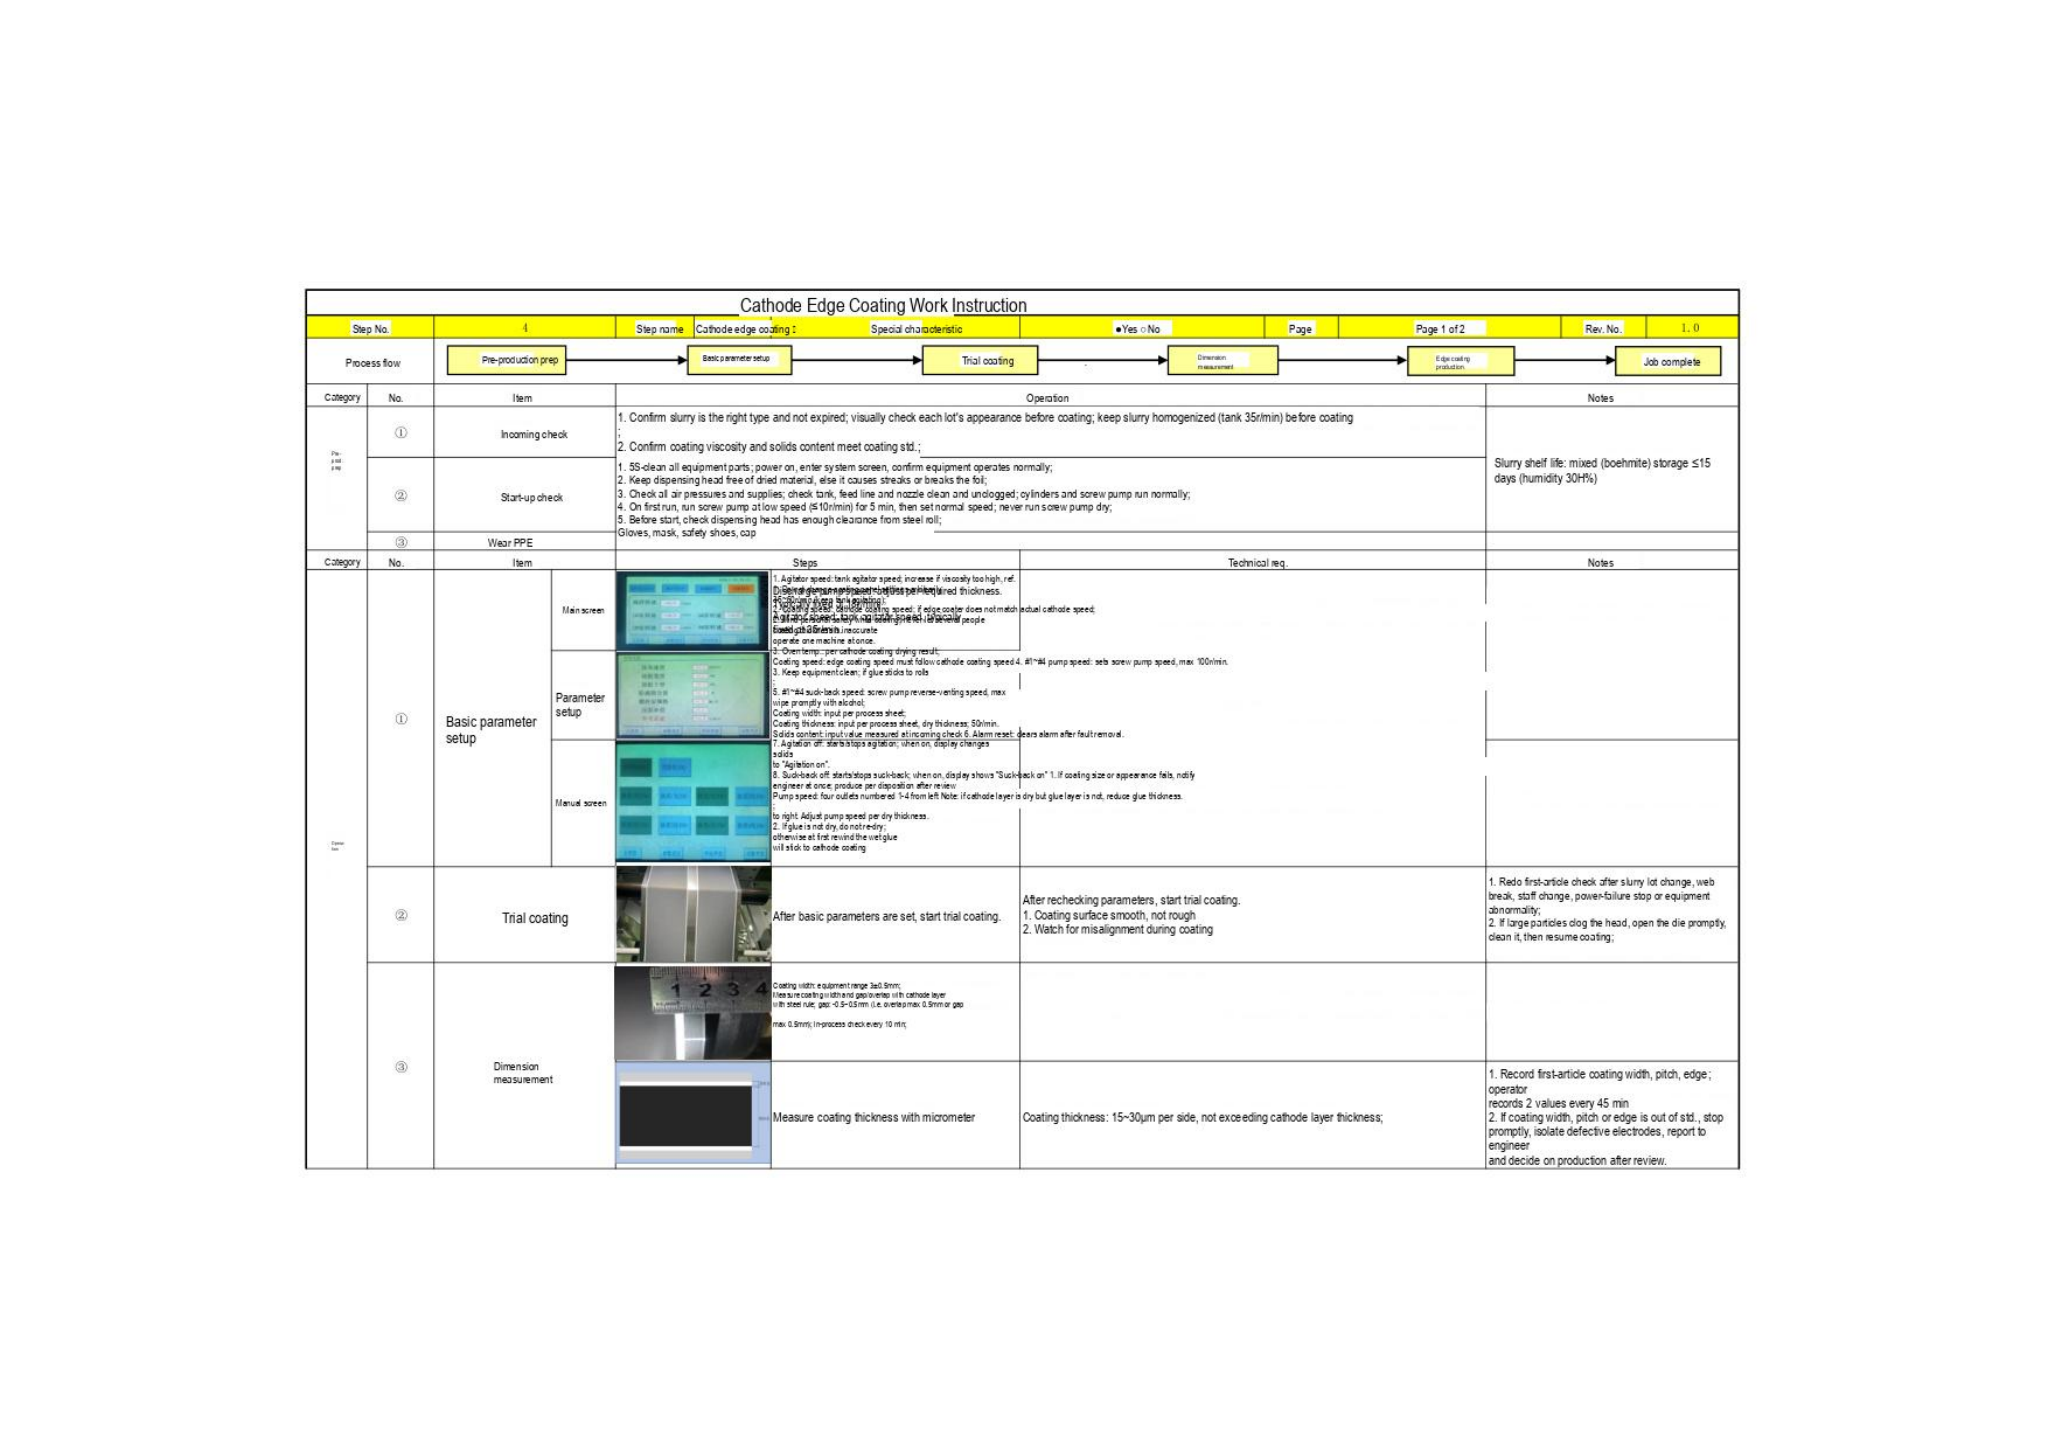# Cathode Edge Coating Work Instruction

| Step No. | 4 | Step name | Cathode edge coating | Special characteristic | ●Yes ○No | Page | Page 1 of 2 | Rev. No. | 1.0 |
|---|---|---|---|---|---|---|---|---|---|

Process flow: Pre-production prep → Basic parameter setup → Trial coating → Dimension measurement → Edge coating production → Job complete

| Category | No. | Item | Operation | Notes |
|---|---|---|---|---|
| Pre-prod prep | ① | Incoming check | 1. Confirm slurry is the right type and not expired; visually check each lot's appearance before coating; keep slurry homogenized (tank 35r/min) before coating<br>;<br>2. Confirm coating viscosity and solids content meet coating std.; | Slurry shelf life: mixed (boehmite) storage ≤15 days (humidity 30H%) |
| | ② | Start-up check | 1. 5S-clean all equipment parts; power on, enter system screen, confirm equipment operates normally;<br>2. Keep dispensing head free of dried material, else it causes streaks or breaks the foil;<br>3. Check all air pressures and supplies; check tank, feed line and nozzle clean and unclogged; cylinders and screw pump run normally;<br>4. On first run, run screw pump at low speed (≤10r/min) for 5 min, then set normal speed; never run screw pump dry;<br>5. Before start, check dispensing head has enough clearance from steel roll; | |
| | ③ | Wear PPE | Gloves, mask, safety shoes, cap | |

| Category | No. | Item | | Steps | Technical req. | Notes |
|---|---|---|---|---|---|---|
| Operation | ① | Basic parameter setup | Main screen<br>Parameter setup<br>Manual screen | 1. Agitator speed: tank agitator speed; increase if viscosity too high, ref.<br>Dispense pump speed: adjust per required thickness.<br>2. Coating speed: cathode coating speed; if edge coater does not match actual cathode speed;<br>inaccurate<br>operate one machine at once.<br>3. Oven temp.: per cathode coating drying result;<br>Coating speed: edge coating speed must follow cathode coating speed 4. #1~#4 pump speed: sets screw pump speed, max 100r/min.<br>3. Keep equipment clean; if glue sticks to rolls<br>5. #1~#4 suck-back speed: screw pump reverse-venting speed, max<br>wipe promptly with alcohol;<br>Coating width: input per process sheet;<br>Coating thickness: input per process sheet, dry thickness; 50r/min.<br>Solids content: input value measured at incoming check 6. Alarm reset: clears alarm after fault removal.<br>7. Agitation off: starts/stops agitation; when on, display changes<br>solids<br>to "Agitation on".<br>8. Suck-back off: starts/stops suck-back; when on, display shows "Suck-back on" 1. If coating size or appearance fails, notify<br>engineer at once; produce per disposition after review<br>Pump speed: four outlets numbered 1-4 from left Note: if cathode layer is dry but glue layer is not, reduce glue thickness.<br>to right. Adjust pump speed per dry thickness.<br>2. If glue is not dry, do not re-dry;<br>otherwise at first rewind the wet glue<br>will stick to cathode coating | | |
| | ② | Trial coating | | After basic parameters are set, start trial coating. | After rechecking parameters, start trial coating.<br>1. Coating surface smooth, not rough<br>2. Watch for misalignment during coating | 1. Redo first-article check after slurry lot change, web break, staff change, power-failure stop or equipment abnormality;<br>2. If large particles clog the head, open the die promptly, clean it, then resume coating; |
| | ③ | Dimension measurement | | 1 2 3 4<br>Coating width: equipment range 3±0.5mm;<br>Measure coating width and gap/overlap with cathode layer with steel rule; gap: -0.5~0.5mm (i.e. overlap max 0.5mm or gap max 0.5mm); in-process check every 10 min; | | |
| | | | | Measure coating thickness with micrometer | Coating thickness: 15~30μm per side, not exceeding cathode layer thickness; | 1. Record first-article coating width, pitch, edge; operator records 2 values every 45 min<br>2. If coating width, pitch or edge is out of std., stop promptly, isolate defective electrodes, report to engineer and decide on production after review. |
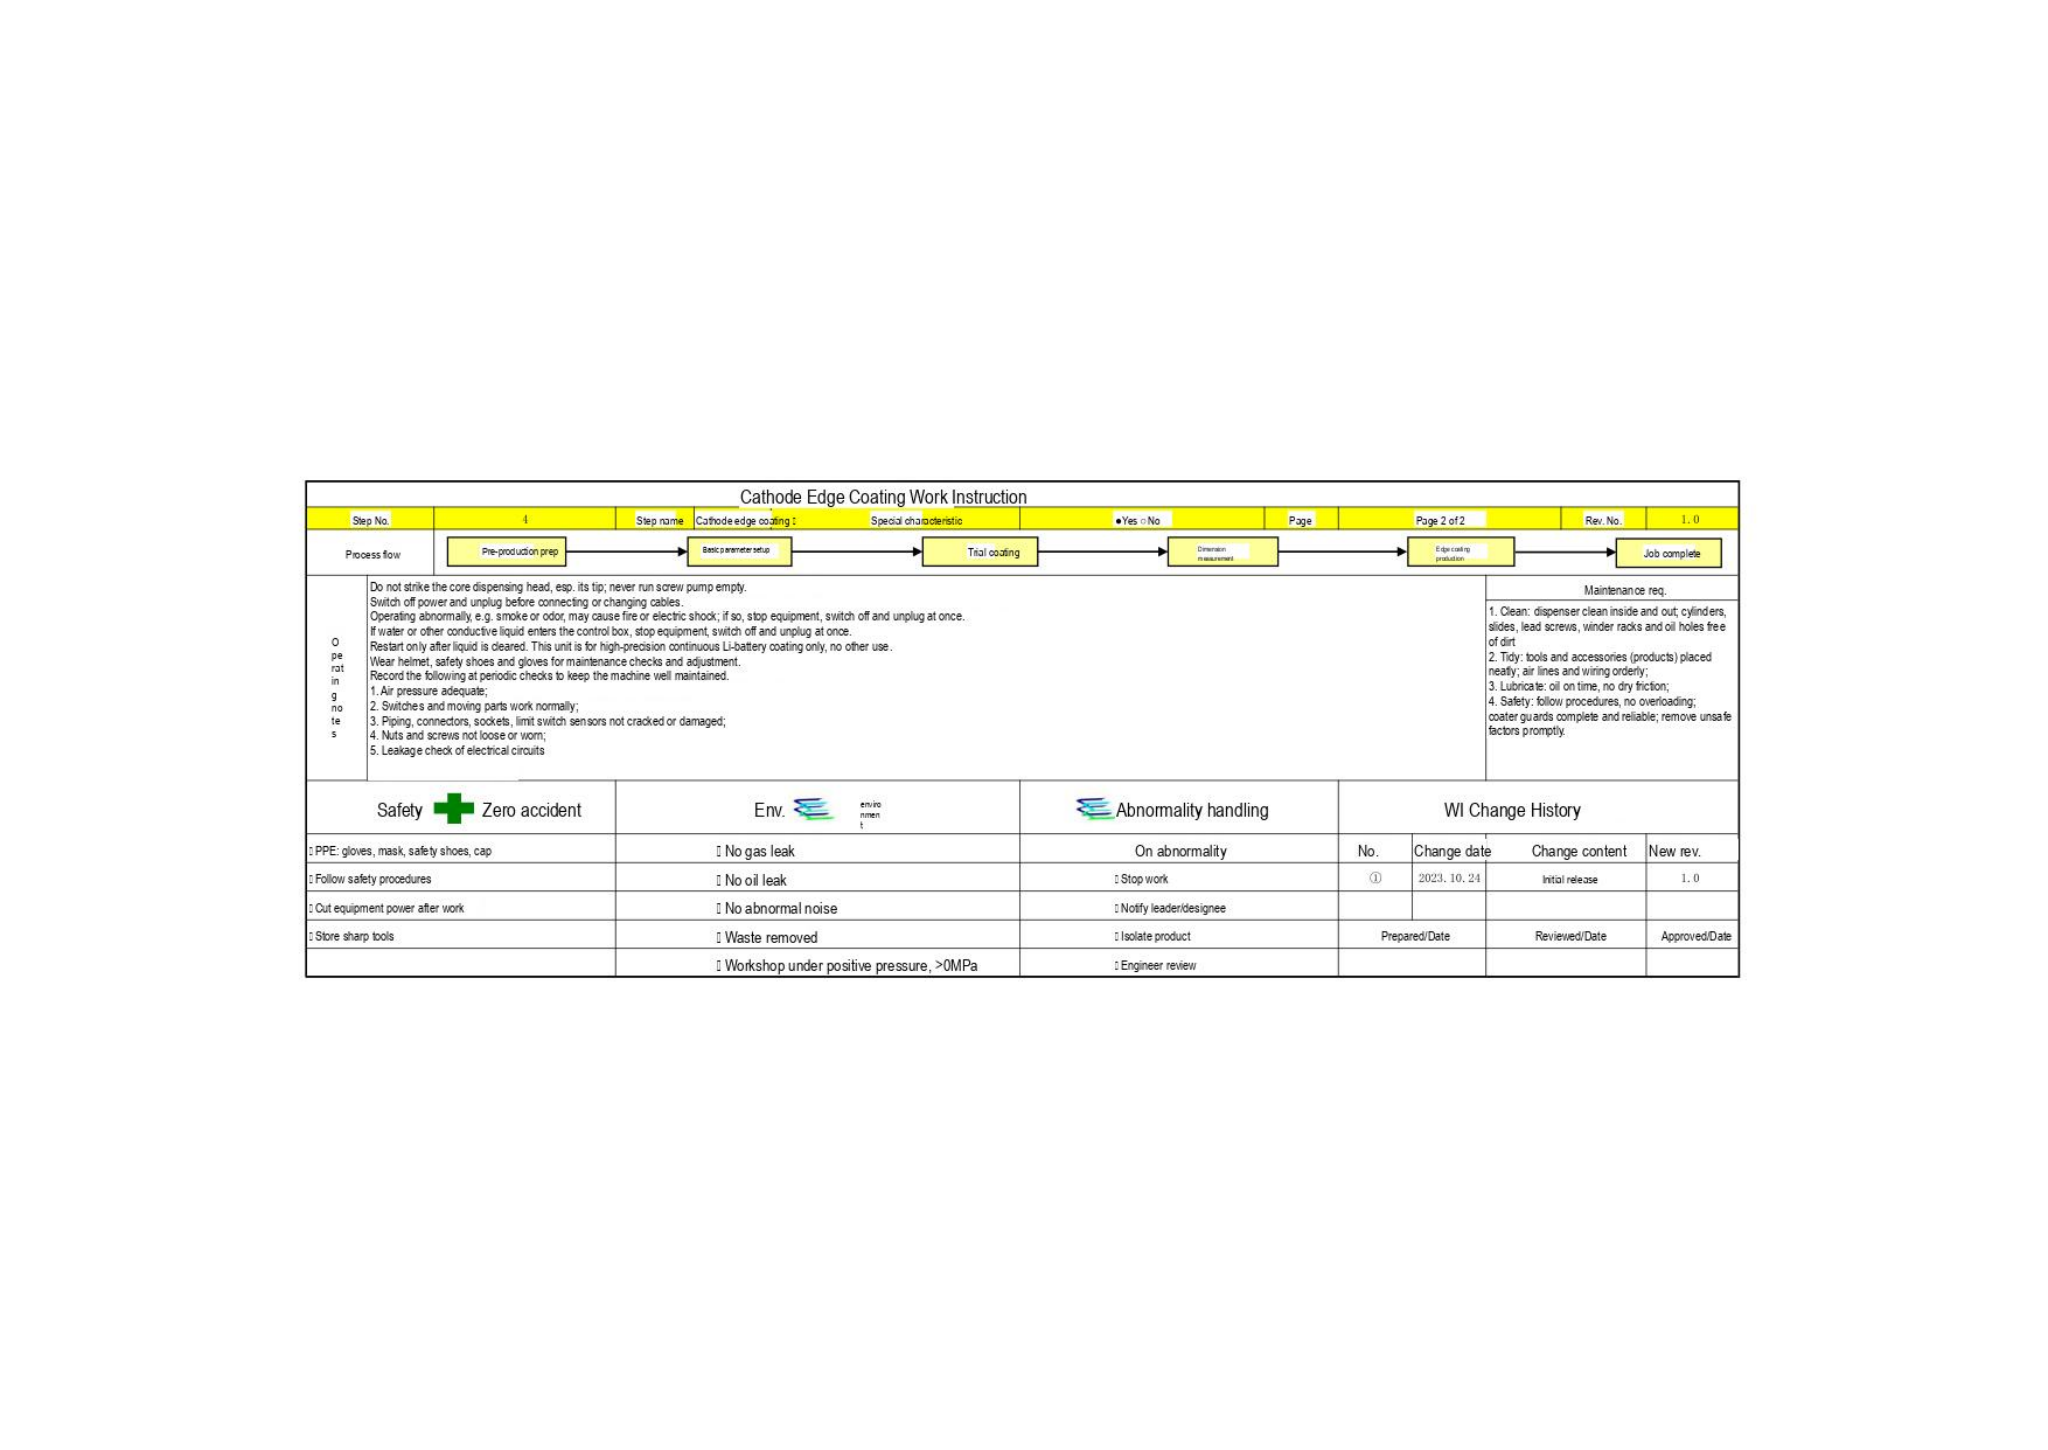Cathode Edge Coating Work Instruction

| Step No. | 4 | Step name | Cathode edge coating | Special characteristic | ●Yes ○No | Page | Page 2 of 2 | Rev. No. | 1.0 |
|---|---|---|---|---|---|---|---|---|---|

Process flow: Pre-production prep → Basic parameter setup → Trial coating → Dimension measurement → Edge coating production → Job complete

Operating notes

Do not strike the core dispensing head, esp. its tip; never run screw pump empty.
Switch off power and unplug before connecting or changing cables.
Operating abnormally, e.g. smoke or odor, may cause fire or electric shock; if so, stop equipment, switch off and unplug at once.
If water or other conductive liquid enters the control box, stop equipment, switch off and unplug at once.
Restart only after liquid is cleared. This unit is for high-precision continuous Li-battery coating only, no other use.
Wear helmet, safety shoes and gloves for maintenance checks and adjustment.
Record the following at periodic checks to keep the machine well maintained.
1. Air pressure adequate;
2. Switches and moving parts work normally;
3. Piping, connectors, sockets, limit switch sensors not cracked or damaged;
4. Nuts and screws not loose or worn;
5. Leakage check of electrical circuits

Maintenance req.

1. Clean: dispenser clean inside and out; cylinders, slides, lead screws, winder racks and oil holes free of dirt
2. Tidy: tools and accessories (products) placed neatly; air lines and wiring orderly;
3. Lubricate: oil on time, no dry friction;
4. Safety: follow procedures, no overloading; coater guards complete and reliable; remove unsafe factors promptly.

| Safety Zero accident | Env. environment | Abnormality handling | WI Change History | | | |
|---|---|---|---|---|---|---|
| PPE: gloves, mask, safety shoes, cap | No gas leak | On abnormality | No. | Change date | Change content | New rev. |
| Follow safety procedures | No oil leak | Stop work | ① | 2023.10.24 | Initial release | 1.0 |
| Cut equipment power after work | No abnormal noise | Notify leader/designee | | | | |
| Store sharp tools | Waste removed | Isolate product | Prepared/Date | | Reviewed/Date | Approved/Date |
| | Workshop under positive pressure, >0MPa | Engineer review | | | | |